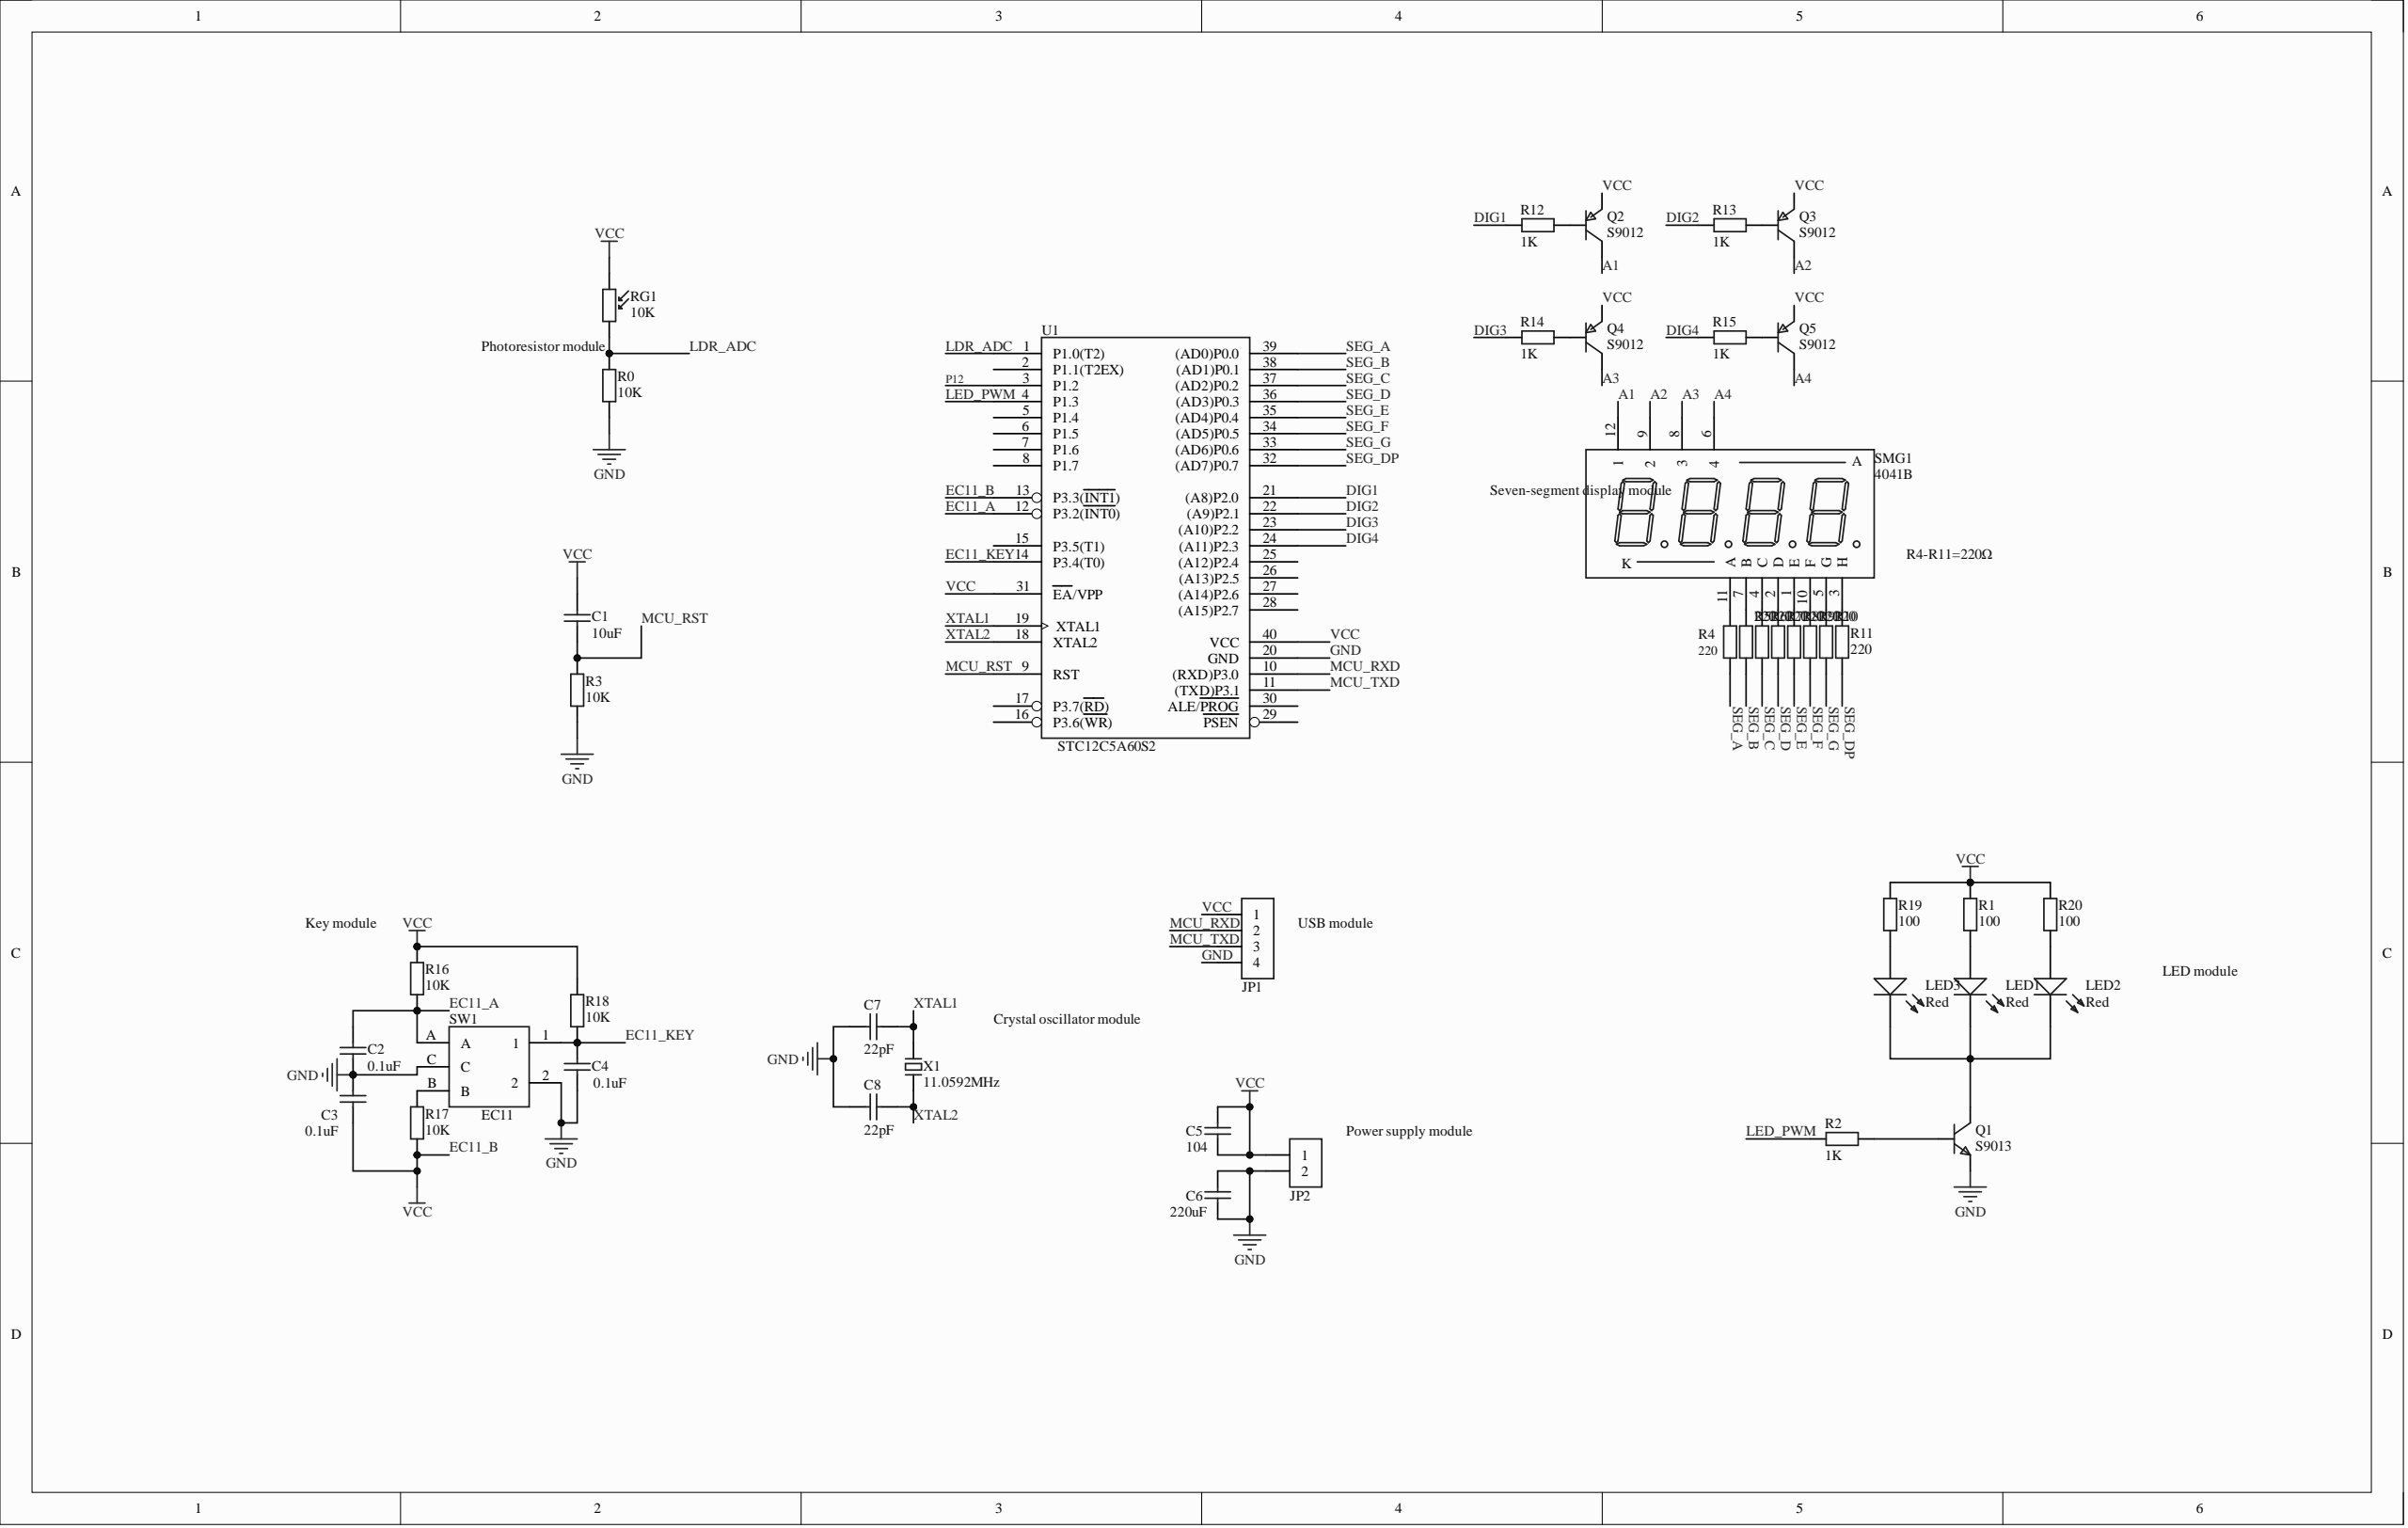Circuit board | Altium Designer | 44 parts | 45 nets
Bill of materials:
Comment,Description,Designator,Footprint,LibRef,Quantity
"10uF","SMD capacitor/MLCC","C1","C0805_L","10uF","1"
"0.1uF","SMD capacitor/MLCC","C2, C3, C4","C0805_L","0.1uF","3"
"104","Ceramic capacitor","C5","CC 1.8*3.6","104","1"
"220uF","SMD capacitor/MLCC","C6","C0805_L","220uF","1"
"22pF","Ceramic capacitor","C7, C8","CC 1.8*3.6","22pF","2"
"HDR-1X4","4P connector","JP1","XH2.54-LI-4P","HDR-1X4","1"
"HDR-1X2","2P connector","JP2","XH2.54-LI-2P","HDR-1X2","1"
"Red","3mm through-hole LED","LED1, LED2, LED3","LED 3MM-B","红色","3"
"S9013","Low-frequency amplifier, NPN type","Q1","TO92A","S9013","1"
"S9012","Low-frequency amplifier, PNP type","Q2, Q3, Q4, Q5","TO92A","S9012","4"
"10K","SMD resistor","R0, R3, R16, R17, R18","AXIAL0.4-1/4W","10K_1","5"
"100","SMD resistor","R1, R19, R20","AXIAL0.3-1/8W","100","3"
"1K","SMD resistor","R2","AXIAL0.3-1/8W","1K","1"
"220","SMD resistor","R4, R5, R6, R7, R8, R9, R10, R11","AXIAL0.4-1/4W","220","8"
"1K","SMD resistor","R12, R13, R14, R15","AXIAL0.4-1/4W","1K_1","4"
"10K","Photoresistor","RG1","RG5528","10K","1"
"4041B","0.4 inch 4-digit common-anode seven-segment display","SMG1","SMG 0.4-4P","4041B","1"
"EC11","Digital rotary encoder switch","SW1","EC11-B","EC11","1"
"STC12C5A60S2","8-Bit Microcontroller with 8K Flash ROM","U1","DIP-40","STC12C5A60S2","1"
"11.059MHz","2-pin passive crystal oscillator (resonator)","X1","HC-49S","11.059MHz","1"
Netlist (Protel format):
[
C1
C0805_L
10uF



]
[
C2
C0805_L
0.1uF



]
[
C3
C0805_L
0.1uF



]
[
C4
C0805_L
0.1uF



]
[
C5
CC 1.8*3.6
104



]
[
C6
C0805_L
220uF



]
[
C7
CC 1.8*3.6
22pF



]
[
C8
CC 1.8*3.6
22pF



]
[
JP1
XH2.54-LI-4P
HDR-1X4



]
[
JP2
XH2.54-LI-2P
HDR-1X2



]
[
LED1
LED 3MM-B
Red



]
[
LED2
LED 3MM-B
Red



]
[
LED3
LED 3MM-B
Red



]
[
Q1
TO92A
S9013



]
[
Q2
TO92A
S9012



]
[
Q3
TO92A
S9012



]
[
Q4
TO92A
S9012



]
[
Q5
TO92A
S9012



]
[
R0
AXIAL0.4-1/4W
10K



]
[
R1
AXIAL0.3-1/8W
100



]
[
R2
AXIAL0.3-1/8W
1K



]
[
R3
AXIAL0.4-1/4W
10K



]
[
R4
AXIAL0.4-1/4W
220



]
[
R5
AXIAL0.4-1/4W
220



]
[
R6
AXIAL0.4-1/4W
220



]
[
R7
AXIAL0.4-1/4W
220



]
[
R8
AXIAL0.4-1/4W
220



]
[
R9
AXIAL0.4-1/4W
220



]
[
R10
AXIAL0.4-1/4W
220



]
[
R11
AXIAL0.4-1/4W
220



]
[
R12
AXIAL0.4-1/4W
1K



]
[
R13
AXIAL0.4-1/4W
1K



]
[
R14
AXIAL0.4-1/4W
1K



]
[
R15
AXIAL0.4-1/4W
1K



]
[
R16
AXIAL0.4-1/4W
10K



]
[
R17
AXIAL0.4-1/4W
10K



]
[
R18
AXIAL0.4-1/4W
10K



]
[
R19
AXIAL0.3-1/8W
100



]
[
R20
AXIAL0.3-1/8W
100



]
[
RG1
RG5528
10K



]
[
SMG1
SMG 0.4-4P
4041B



]
[
SW1
EC11-B
EC11



]
[
U1
DIP-40
STC12C5A60S2



]
[
X1
HC-49S
11.0592MHz



]
(
XTAL2
C8-2
U1-18
X1-1
)
(
XTAL1
C7-2
U1-19
X1-2
)
(
SEG_G
R10-2
U1-33
)
(
SEG_F
R9-1
U1-34
)
(
SEG_E
R8-1
U1-35
)
(
SEG_DP
R11-1
U1-32
)
(
SEG_D
R7-1
U1-36
)
(
SEG_C
R6-1
U1-37
)
(
SEG_B
R5-1
U1-38
)
(
SEG_A
R4-2
U1-39
)
(
NetR17_2
R17-2
SW1-B
)
(
NetR11_2
R11-2
SMG1-3
)
(
NetR10_1
R10-1
SMG1-5
)
(
NetR9_2
R9-2
SMG1-10
)
(
NetR8_2
R8-2
SMG1-1
)
(
NetR7_2
R7-2
SMG1-2
)
(
NetR6_2
R6-2
SMG1-4
)
(
NetR5_2
R5-2
SMG1-7
)
(
NetR4_1
R4-1
SMG1-11
)
(
NetQ5_2
Q5-2
R15-2
)
(
NetQ4_2
Q4-2
R14-2
)
(
NetQ3_2
Q3-2
R13-2
)
(
NetQ2_2
Q2-2
R12-2
)
(
NetQ1_2
Q1-2
R2-2
)
(
NetLED3_1
LED3-1
R19-1
)
(
NetLED2_1
LED2-1
R20-1
)
(
NetLED1_2
LED1-2
LED2-2
LED3-2
Q1-3
)
(
NetLED1_1
LED1-1
R1-1
)
(
MCU_TXD
JP1-3
U1-11
)
(
MCU_RXD
JP1-2
U1-10
)
(
MCU_RST
C1-1
R3-1
U1-9
)
(
LED_PWM
R2-1
U1-4
)
(
LDR_ADC
R0-1
RG1-2
U1-1
)
(
GND
C2-1
C3-2
C4-1
C6-1
C6-2
C7-1
C8-1
JP1-4
JP2-2
Q1-1
R0-2
R3-2
SW1-2
SW1-C
U1-20
)
(
EC11_KEY
C4-2
R18-1
SW1-1
U1-14
)
(
EC11_B
C1-2
C3-1
C5-1
C5-2
JP1-1
JP2-1
Q2-1
Q3-1
Q4-1
Q5-1
R1-2
R16-2
R17-1
R18-2
R19-2
R20-2
RG1-1
U1-13
U1-31
U1-40
)
(
EC11_A
C2-2
R16-1
SW1-A
U1-12
)
(
DIG4
R15-1
U1-24
)
(
DIG3
R14-1
U1-23
)
(
DIG2
R13-1
U1-22
)
(
DIG1
R12-1
U1-21
)
(
A4
Q5-3
SMG1-6
)
(
A3
Q4-3
SMG1-8
)
(
A2
Q3-3
SMG1-9
)
(
A1
Q2-3
SMG1-12
)